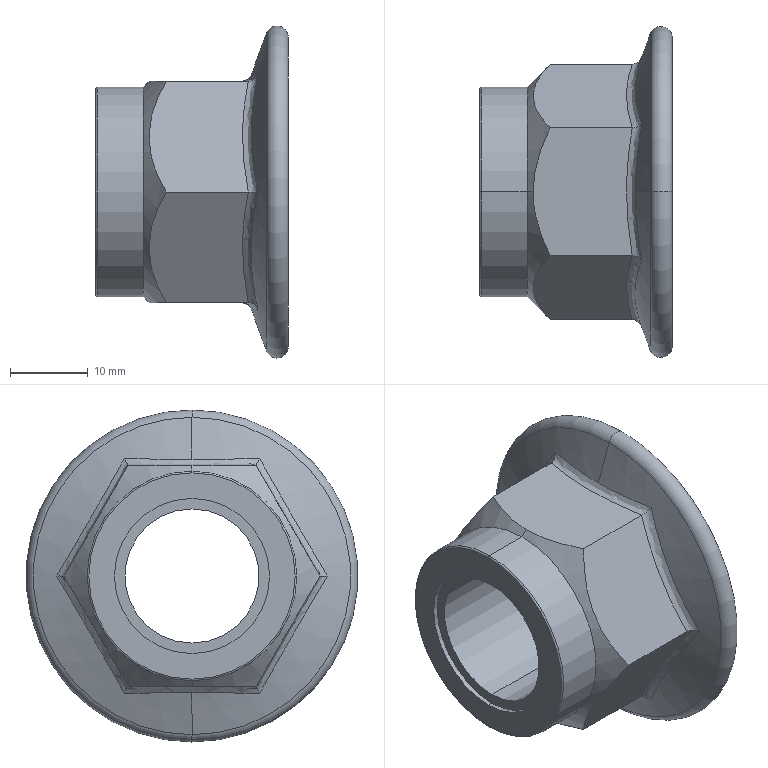Part | SolidWorks | features Cut 2, Revolution 2, Boss 1, Chamfer 1, Fillet 1 | 1 solid | 31 faces | box 24.8 x 42.8 x 42.8 mm | volume 13100 mm3 | plane 9 | cylinder 6 | cone 6 | spline 6 | torus 4 | commonest cylinder face diameters 17.294 x2 20 x2 27 x2
STEP:
#1=CARTESIAN_POINT('',(-24.8,0.,10.));
#2=VERTEX_POINT('',#1);
#3=CARTESIAN_POINT('',(-24.8,0.,-10.));
#4=VERTEX_POINT('',#3);
#5=CARTESIAN_POINT('',(-24.8,0.,0.));
#6=DIRECTION('',(1.,0.,0.));
#7=DIRECTION('',(0.,0.,-1.));
#8=AXIS2_PLACEMENT_3D('',#5,#6,#7);
#9=CIRCLE('',#8,10.);
#10=EDGE_CURVE('',#2,#4,#9,.T.);
#11=ORIENTED_EDGE('',*,*,#10,.F.);
#12=CARTESIAN_POINT('',(-24.19,0.,10.));
#13=VERTEX_POINT('',#12);
#14=CARTESIAN_POINT('',(0.,0.,10.));
#15=DIRECTION('',(1.,0.,0.));
#16=VECTOR('',#15,1000.);
#17=LINE('',#14,#16);
#18=EDGE_CURVE('',#2,#13,#17,.T.);
#19=ORIENTED_EDGE('',*,*,#18,.T.);
#20=CARTESIAN_POINT('',(-24.19,0.,-10.));
#21=VERTEX_POINT('',#20);
#22=CARTESIAN_POINT('',(-24.19,0.,0.));
#23=DIRECTION('',(1.,0.,0.));
#24=DIRECTION('',(0.,0.,-1.));
#25=AXIS2_PLACEMENT_3D('',#22,#23,#24);
#26=CIRCLE('',#25,10.);
#27=EDGE_CURVE('',#13,#21,#26,.T.);
#28=ORIENTED_EDGE('',*,*,#27,.T.);
#29=CARTESIAN_POINT('',(0.,0.,-10.));
#30=DIRECTION('',(1.,0.,0.));
#31=VECTOR('',#30,1000.);
#32=LINE('',#29,#31);
#33=EDGE_CURVE('',#4,#21,#32,.T.);
#34=ORIENTED_EDGE('',*,*,#33,.F.);
#35=EDGE_LOOP('',(#11,#19,#28,#34));
#36=FACE_OUTER_BOUND('',#35,.T.);
#37=CARTESIAN_POINT('',(0.,0.,0.));
#38=DIRECTION('',(1.,0.,0.));
#39=DIRECTION('',(0.,0.,-1.));
#40=AXIS2_PLACEMENT_3D('',#37,#38,#39);
#41=CYLINDRICAL_SURFACE('',#40,10.);
#42=ADVANCED_FACE('',(#36),#41,.F.);
#43=CARTESIAN_POINT('',(-24.8,0.,-13.3));
#44=VERTEX_POINT('',#43);
#45=CARTESIAN_POINT('',(-24.8,0.,13.3));
#46=VERTEX_POINT('',#45);
#47=CARTESIAN_POINT('',(-24.8,0.,0.));
#48=DIRECTION('',(1.,0.,0.));
#49=DIRECTION('',(0.,0.,-1.));
#50=AXIS2_PLACEMENT_3D('',#47,#48,#49);
#51=CIRCLE('',#50,13.3);
#52=EDGE_CURVE('',#44,#46,#51,.T.);
#53=ORIENTED_EDGE('',*,*,#52,.T.);
#54=CARTESIAN_POINT('',(-24.6,0.,13.5));
#55=VERTEX_POINT('',#54);
#56=CARTESIAN_POINT('',(-24.6,0.,13.3));
#57=DIRECTION('',(0.,1.,0.));
#58=DIRECTION('',(0.,0.,1.));
#59=AXIS2_PLACEMENT_3D('',#56,#57,#58);
#60=CIRCLE('',#59,0.2);
#61=EDGE_CURVE('',#46,#55,#60,.T.);
#62=ORIENTED_EDGE('',*,*,#61,.T.);
#63=CARTESIAN_POINT('',(-24.6,0.,-13.5));
#64=VERTEX_POINT('',#63);
#65=CARTESIAN_POINT('',(-24.6,0.,0.));
#66=DIRECTION('',(1.,0.,0.));
#67=DIRECTION('',(0.,0.,-1.));
#68=AXIS2_PLACEMENT_3D('',#65,#66,#67);
#69=CIRCLE('',#68,13.5);
#70=EDGE_CURVE('',#64,#55,#69,.T.);
#71=ORIENTED_EDGE('',*,*,#70,.F.);
#72=CARTESIAN_POINT('',(-24.6,0.,-13.3));
#73=DIRECTION('',(0.,-1.,0.));
#74=DIRECTION('',(0.,0.,-1.));
#75=AXIS2_PLACEMENT_3D('',#72,#73,#74);
#76=CIRCLE('',#75,0.2);
#77=EDGE_CURVE('',#44,#64,#76,.T.);
#78=ORIENTED_EDGE('',*,*,#77,.F.);
#79=EDGE_LOOP('',(#53,#62,#71,#78));
#80=FACE_OUTER_BOUND('',#79,.T.);
#81=CARTESIAN_POINT('',(-24.6,0.,0.));
#82=DIRECTION('',(1.,0.,0.));
#83=DIRECTION('',(0.,0.,-1.));
#84=AXIS2_PLACEMENT_3D('',#81,#82,#83);
#85=TOROIDAL_SURFACE('',#84,13.3,0.2);
#86=ADVANCED_FACE('',(#80),#85,.T.);
#87=ORIENTED_EDGE('',*,*,#70,.T.);
#88=CARTESIAN_POINT('',(-18.7,0.,13.5));
#89=VERTEX_POINT('',#88);
#90=CARTESIAN_POINT('',(0.,0.,13.5));
#91=DIRECTION('',(1.,0.,0.));
#92=VECTOR('',#91,1000.);
#93=LINE('',#90,#92);
#94=EDGE_CURVE('',#55,#89,#93,.T.);
#95=ORIENTED_EDGE('',*,*,#94,.T.);
#96=CARTESIAN_POINT('',(-18.7,0.,-13.5));
#97=VERTEX_POINT('',#96);
#98=CARTESIAN_POINT('',(-18.7,0.,0.));
#99=DIRECTION('',(-1.,0.,0.));
#100=DIRECTION('',(0.,0.,1.));
#101=AXIS2_PLACEMENT_3D('',#98,#99,#100);
#102=CIRCLE('',#101,13.5);
#103=EDGE_CURVE('',#89,#97,#102,.T.);
#104=ORIENTED_EDGE('',*,*,#103,.T.);
#105=CARTESIAN_POINT('',(0.,0.,-13.5));
#106=DIRECTION('',(1.,0.,0.));
#107=VECTOR('',#106,1000.);
#108=LINE('',#105,#107);
#109=EDGE_CURVE('',#64,#97,#108,.T.);
#110=ORIENTED_EDGE('',*,*,#109,.F.);
#111=EDGE_LOOP('',(#87,#95,#104,#110));
#112=FACE_OUTER_BOUND('',#111,.T.);
#113=CARTESIAN_POINT('',(0.,0.,0.));
#114=DIRECTION('',(1.,0.,0.));
#115=DIRECTION('',(0.,0.,-1.));
#116=AXIS2_PLACEMENT_3D('',#113,#114,#115);
#117=CYLINDRICAL_SURFACE('',#116,13.5);
#118=ADVANCED_FACE('',(#112),#117,.T.);
#119=CARTESIAN_POINT('',(-18.7,0.,0.));
#120=DIRECTION('',(-1.,0.,0.));
#121=DIRECTION('',(0.,0.,1.));
#122=AXIS2_PLACEMENT_3D('',#119,#120,#121);
#123=CIRCLE('',#122,13.5);
#124=EDGE_CURVE('',#97,#89,#123,.T.);
#125=ORIENTED_EDGE('',*,*,#124,.F.);
#126=CARTESIAN_POINT('',(-17.932,0.,-14.268));
#127=VERTEX_POINT('',#126);
#128=CARTESIAN_POINT('',(-18.7,0.,-13.5));
#129=DIRECTION('',(0.7071,0.,-0.7071));
#130=VECTOR('',#129,1000.);
#131=LINE('',#128,#130);
#132=EDGE_CURVE('',#97,#127,#131,.T.);
#133=ORIENTED_EDGE('',*,*,#132,.T.);
#134=CARTESIAN_POINT('',(-15.725,-8.238,-14.268));
#135=VERTEX_POINT('',#134);
#136=CARTESIAN_POINT('',(-17.932,0.,-14.268));
#137=CARTESIAN_POINT('',(-17.932,-0.3616,-14.268));
#138=CARTESIAN_POINT('',(-17.918,-0.7252,-14.268));
#139=CARTESIAN_POINT('',(-17.864,-1.443,-14.268));
#140=CARTESIAN_POINT('',(-17.824,-1.799,-14.268));
#141=CARTESIAN_POINT('',(-17.665,-2.859,-14.268));
#142=CARTESIAN_POINT('',(-17.511,-3.555,-14.268));
#143=CARTESIAN_POINT('',(-17.119,-4.928,-14.268));
#144=CARTESIAN_POINT('',(-16.882,-5.607,-14.268));
#145=CARTESIAN_POINT('',(-16.343,-6.947,-14.268));
#146=CARTESIAN_POINT('',(-16.044,-7.599,-14.268));
#147=CARTESIAN_POINT('',(-15.725,-8.238,-14.268));
#148=B_SPLINE_CURVE_WITH_KNOTS('',3,(#136,#137,#138,#139,#140,#141,#142,#143,#144,#145,#146,#147),.UNSPECIFIED.,.F.,.F.,(4,2,2,2,2,4),(0.01727,0.01833,0.0194,0.02153,0.02366,0.0258),.UNSPECIFIED.);
#149=EDGE_CURVE('',#127,#135,#148,.T.);
#150=ORIENTED_EDGE('',*,*,#149,.T.);
#151=CARTESIAN_POINT('',(-15.725,-16.475,0.));
#152=VERTEX_POINT('',#151);
#153=CARTESIAN_POINT('',(-15.725,-8.238,-14.268));
#154=CARTESIAN_POINT('',(-16.369,-8.881,-13.153));
#155=CARTESIAN_POINT('',(-16.916,-9.539,-12.013));
#156=CARTESIAN_POINT('',(-17.502,-10.562,-10.242));
#157=CARTESIAN_POINT('',(-17.658,-10.909,-9.641));
#158=CARTESIAN_POINT('',(-17.873,-11.617,-8.415));
#159=CARTESIAN_POINT('',(-17.931,-11.982,-7.783));
#160=CARTESIAN_POINT('',(-17.935,-13.06,-5.915));
#161=CARTESIAN_POINT('',(-17.717,-13.767,-4.69));
#162=CARTESIAN_POINT('',(-16.928,-15.161,-2.276));
#163=CARTESIAN_POINT('',(-16.372,-15.828,-1.121));
#164=CARTESIAN_POINT('',(-15.725,-16.475,0.));
#165=B_SPLINE_CURVE_WITH_KNOTS('',3,(#153,#154,#155,#156,#157,#158,#159,#160,#161,#162,#163,#164),.UNSPECIFIED.,.F.,.F.,(4,2,2,2,2,4),(0.000000254,0.004255,0.006382,0.008509,0.01276,0.01702),.UNSPECIFIED.);
#166=EDGE_CURVE('',#135,#152,#165,.T.);
#167=ORIENTED_EDGE('',*,*,#166,.T.);
#168=CARTESIAN_POINT('',(-15.725,-8.238,14.268));
#169=VERTEX_POINT('',#168);
#170=CARTESIAN_POINT('',(-15.725,-16.475,0.));
#171=CARTESIAN_POINT('',(-16.369,-15.831,1.115));
#172=CARTESIAN_POINT('',(-16.916,-15.173,2.255));
#173=CARTESIAN_POINT('',(-17.502,-14.151,4.026));
#174=CARTESIAN_POINT('',(-17.658,-13.804,4.626));
#175=CARTESIAN_POINT('',(-17.873,-13.096,5.853));
#176=CARTESIAN_POINT('',(-17.931,-12.731,6.485));
#177=CARTESIAN_POINT('',(-17.935,-11.652,8.353));
#178=CARTESIAN_POINT('',(-17.717,-10.945,9.577));
#179=CARTESIAN_POINT('',(-16.928,-9.552,11.992));
#180=CARTESIAN_POINT('',(-16.372,-8.885,13.146));
#181=CARTESIAN_POINT('',(-15.725,-8.238,14.268));
#182=B_SPLINE_CURVE_WITH_KNOTS('',3,(#170,#171,#172,#173,#174,#175,#176,#177,#178,#179,#180,#181),.UNSPECIFIED.,.F.,.F.,(4,2,2,2,2,4),(0.000000254,0.004255,0.006382,0.008509,0.01276,0.01702),.UNSPECIFIED.);
#183=EDGE_CURVE('',#152,#169,#182,.T.);
#184=ORIENTED_EDGE('',*,*,#183,.T.);
#185=CARTESIAN_POINT('',(-17.932,0.,14.268));
#186=VERTEX_POINT('',#185);
#187=CARTESIAN_POINT('',(-15.725,-8.238,14.268));
#188=CARTESIAN_POINT('',(-16.044,-7.599,14.268));
#189=CARTESIAN_POINT('',(-16.343,-6.947,14.268));
#190=CARTESIAN_POINT('',(-16.882,-5.607,14.268));
#191=CARTESIAN_POINT('',(-17.119,-4.928,14.268));
#192=CARTESIAN_POINT('',(-17.511,-3.555,14.268));
#193=CARTESIAN_POINT('',(-17.665,-2.859,14.268));
#194=CARTESIAN_POINT('',(-17.824,-1.799,14.268));
#195=CARTESIAN_POINT('',(-17.864,-1.443,14.268));
#196=CARTESIAN_POINT('',(-17.918,-0.7252,14.268));
#197=CARTESIAN_POINT('',(-17.932,-0.3616,14.268));
#198=CARTESIAN_POINT('',(-17.932,0.,14.268));
#199=B_SPLINE_CURVE_WITH_KNOTS('',3,(#187,#188,#189,#190,#191,#192,#193,#194,#195,#196,#197,#198),.UNSPECIFIED.,.F.,.F.,(4,2,2,2,2,4),(0.01093,0.01306,0.0152,0.01733,0.0184,0.01946),.UNSPECIFIED.);
#200=EDGE_CURVE('',#169,#186,#199,.T.);
#201=ORIENTED_EDGE('',*,*,#200,.T.);
#202=CARTESIAN_POINT('',(-18.7,0.,13.5));
#203=DIRECTION('',(0.7071,0.,0.7071));
#204=VECTOR('',#203,1000.);
#205=LINE('',#202,#204);
#206=EDGE_CURVE('',#89,#186,#205,.T.);
#207=ORIENTED_EDGE('',*,*,#206,.F.);
#208=EDGE_LOOP('',(#125,#133,#150,#167,#184,#201,#207));
#209=FACE_OUTER_BOUND('',#208,.T.);
#210=CARTESIAN_POINT('',(-18.7,0.,0.));
#211=DIRECTION('',(1.,0.,0.));
#212=DIRECTION('',(0.,0.,1.));
#213=AXIS2_PLACEMENT_3D('',#210,#211,#212);
#214=CONICAL_SURFACE('',#213,13.5,0.7854);
#215=ADVANCED_FACE('',(#209),#214,.T.);
#216=CARTESIAN_POINT('',(-2.153,0.,8.647));
#217=VERTEX_POINT('',#216);
#218=CARTESIAN_POINT('',(-2.153,0.,-8.647));
#219=VERTEX_POINT('',#218);
#220=CARTESIAN_POINT('',(-2.153,0.,0.));
#221=DIRECTION('',(1.,0.,0.));
#222=DIRECTION('',(0.,0.,1.));
#223=AXIS2_PLACEMENT_3D('',#220,#221,#222);
#224=CIRCLE('',#223,8.647);
#225=EDGE_CURVE('',#217,#219,#224,.T.);
#226=ORIENTED_EDGE('',*,*,#225,.F.);
#227=CARTESIAN_POINT('',(0.,0.,10.8));
#228=VERTEX_POINT('',#227);
#229=CARTESIAN_POINT('',(0.,0.,10.8));
#230=DIRECTION('',(0.7071,0.,0.7071));
#231=VECTOR('',#230,1000.);
#232=LINE('',#229,#231);
#233=EDGE_CURVE('',#217,#228,#232,.T.);
#234=ORIENTED_EDGE('',*,*,#233,.T.);
#235=CARTESIAN_POINT('',(0.,0.,-10.8));
#236=VERTEX_POINT('',#235);
#237=CARTESIAN_POINT('',(0.,0.,0.));
#238=DIRECTION('',(-1.,0.,0.));
#239=DIRECTION('',(0.,0.,1.));
#240=AXIS2_PLACEMENT_3D('',#237,#238,#239);
#241=CIRCLE('',#240,10.8);
#242=EDGE_CURVE('',#236,#228,#241,.T.);
#243=ORIENTED_EDGE('',*,*,#242,.F.);
#244=CARTESIAN_POINT('',(0.,0.,-10.8));
#245=DIRECTION('',(0.7071,0.,-0.7071));
#246=VECTOR('',#245,1000.);
#247=LINE('',#244,#246);
#248=EDGE_CURVE('',#219,#236,#247,.T.);
#249=ORIENTED_EDGE('',*,*,#248,.F.);
#250=EDGE_LOOP('',(#226,#234,#243,#249));
#251=FACE_OUTER_BOUND('',#250,.T.);
#252=CARTESIAN_POINT('',(0.,0.,0.));
#253=DIRECTION('',(1.,0.,0.));
#254=DIRECTION('',(0.,0.,-1.));
#255=AXIS2_PLACEMENT_3D('',#252,#253,#254);
#256=CONICAL_SURFACE('',#255,10.8,0.7854);
#257=ADVANCED_FACE('',(#251),#256,.F.);
#258=ORIENTED_EDGE('',*,*,#225,.T.);
#259=CARTESIAN_POINT('',(-24.19,0.,-8.647));
#260=VERTEX_POINT('',#259);
#261=CARTESIAN_POINT('',(0.,0.,-8.647));
#262=DIRECTION('',(-1.,0.,0.));
#263=VECTOR('',#262,1000.);
#264=LINE('',#261,#263);
#265=EDGE_CURVE('',#219,#260,#264,.T.);
#266=ORIENTED_EDGE('',*,*,#265,.T.);
#267=CARTESIAN_POINT('',(-24.19,0.,8.647));
#268=VERTEX_POINT('',#267);
#269=CARTESIAN_POINT('',(-24.19,0.,0.));
#270=DIRECTION('',(1.,0.,0.));
#271=DIRECTION('',(0.,0.,-1.));
#272=AXIS2_PLACEMENT_3D('',#269,#270,#271);
#273=CIRCLE('',#272,8.647);
#274=EDGE_CURVE('',#268,#260,#273,.T.);
#275=ORIENTED_EDGE('',*,*,#274,.F.);
#276=CARTESIAN_POINT('',(0.,0.,8.647));
#277=DIRECTION('',(-1.,0.,0.));
#278=VECTOR('',#277,1000.);
#279=LINE('',#276,#278);
#280=EDGE_CURVE('',#217,#268,#279,.T.);
#281=ORIENTED_EDGE('',*,*,#280,.F.);
#282=EDGE_LOOP('',(#258,#266,#275,#281));
#283=FACE_OUTER_BOUND('',#282,.T.);
#284=CARTESIAN_POINT('',(0.,0.,0.));
#285=DIRECTION('',(-1.,0.,0.));
#286=DIRECTION('',(0.,0.,1.));
#287=AXIS2_PLACEMENT_3D('',#284,#285,#286);
#288=CYLINDRICAL_SURFACE('',#287,8.647);
#289=ADVANCED_FACE('',(#283),#288,.F.);
#290=CARTESIAN_POINT('',(0.,0.,19.95));
#291=VERTEX_POINT('',#290);
#292=CARTESIAN_POINT('',(0.,0.,-19.95));
#293=VERTEX_POINT('',#292);
#294=CARTESIAN_POINT('',(0.,0.,0.));
#295=DIRECTION('',(-1.,0.,0.));
#296=DIRECTION('',(0.,0.,1.));
#297=AXIS2_PLACEMENT_3D('',#294,#295,#296);
#298=CIRCLE('',#297,19.95);
#299=EDGE_CURVE('',#291,#293,#298,.T.);
#300=ORIENTED_EDGE('',*,*,#299,.T.);
#301=CARTESIAN_POINT('',(-2.813,0.,-20.446));
#302=VERTEX_POINT('',#301);
#303=CARTESIAN_POINT('',(-1.45,0.,-19.95));
#304=DIRECTION('',(0.,1.,0.));
#305=DIRECTION('',(0.,0.,1.));
#306=AXIS2_PLACEMENT_3D('',#303,#304,#305);
#307=CIRCLE('',#306,1.45);
#308=EDGE_CURVE('',#293,#302,#307,.T.);
#309=ORIENTED_EDGE('',*,*,#308,.T.);
#310=CARTESIAN_POINT('',(-2.813,0.,20.446));
#311=VERTEX_POINT('',#310);
#312=CARTESIAN_POINT('',(-2.813,0.,0.));
#313=DIRECTION('',(-1.,0.,0.));
#314=DIRECTION('',(0.,0.,1.));
#315=AXIS2_PLACEMENT_3D('',#312,#313,#314);
#316=CIRCLE('',#315,20.446);
#317=EDGE_CURVE('',#311,#302,#316,.T.);
#318=ORIENTED_EDGE('',*,*,#317,.F.);
#319=CARTESIAN_POINT('',(-1.45,0.,19.95));
#320=DIRECTION('',(0.,-1.,0.));
#321=DIRECTION('',(0.,0.,-1.));
#322=AXIS2_PLACEMENT_3D('',#319,#320,#321);
#323=CIRCLE('',#322,1.45);
#324=EDGE_CURVE('',#291,#311,#323,.T.);
#325=ORIENTED_EDGE('',*,*,#324,.F.);
#326=EDGE_LOOP('',(#300,#309,#318,#325));
#327=FACE_OUTER_BOUND('',#326,.T.);
#328=CARTESIAN_POINT('',(-1.45,0.,0.));
#329=DIRECTION('',(-1.,0.,0.));
#330=DIRECTION('',(0.,0.,1.));
#331=AXIS2_PLACEMENT_3D('',#328,#329,#330);
#332=TOROIDAL_SURFACE('',#331,19.95,1.45);
#333=ADVANCED_FACE('',(#327),#332,.T.);
#334=CARTESIAN_POINT('',(-3.903,8.725,15.112));
#335=VERTEX_POINT('',#334);
#336=CARTESIAN_POINT('',(-4.774,0.,15.057));
#337=VERTEX_POINT('',#336);
#338=CARTESIAN_POINT('',(-3.903,8.725,15.112));
#339=CARTESIAN_POINT('',(-4.17,7.283,15.098));
#340=CARTESIAN_POINT('',(-4.389,5.836,15.084));
#341=CARTESIAN_POINT('',(-4.692,2.929,15.063));
#342=CARTESIAN_POINT('',(-4.774,1.469,15.057));
#343=CARTESIAN_POINT('',(-4.774,0.,15.057));
#344=B_SPLINE_CURVE_WITH_KNOTS('',3,(#338,#339,#340,#341,#342,#343),.UNSPECIFIED.,.F.,.F.,(4,2,4),(0.,0.004384,0.008769),.UNSPECIFIED.);
#345=EDGE_CURVE('',#335,#337,#344,.T.);
#346=ORIENTED_EDGE('',*,*,#345,.T.);
#347=CARTESIAN_POINT('',(-2.813,0.,20.446));
#348=DIRECTION('',(0.342,0.,0.9397));
#349=VECTOR('',#348,1000.);
#350=LINE('',#347,#349);
#351=EDGE_CURVE('',#337,#311,#350,.T.);
#352=ORIENTED_EDGE('',*,*,#351,.T.);
#353=ORIENTED_EDGE('',*,*,#317,.T.);
#354=CARTESIAN_POINT('',(-4.774,0.,-15.057));
#355=VERTEX_POINT('',#354);
#356=CARTESIAN_POINT('',(-2.813,0.,-20.446));
#357=DIRECTION('',(0.342,0.,-0.9397));
#358=VECTOR('',#357,1000.);
#359=LINE('',#356,#358);
#360=EDGE_CURVE('',#355,#302,#359,.T.);
#361=ORIENTED_EDGE('',*,*,#360,.F.);
#362=CARTESIAN_POINT('',(-3.903,8.725,-15.112));
#363=VERTEX_POINT('',#362);
#364=CARTESIAN_POINT('',(-4.774,0.,-15.057));
#365=CARTESIAN_POINT('',(-4.774,1.465,-15.057));
#366=CARTESIAN_POINT('',(-4.692,2.925,-15.063));
#367=CARTESIAN_POINT('',(-4.389,5.839,-15.084));
#368=CARTESIAN_POINT('',(-4.17,7.285,-15.098));
#369=CARTESIAN_POINT('',(-3.903,8.725,-15.112));
#370=B_SPLINE_CURVE_WITH_KNOTS('',3,(#364,#365,#366,#367,#368,#369),.UNSPECIFIED.,.F.,.F.,(4,2,4),(0.008769,0.01314,0.01751),.UNSPECIFIED.);
#371=EDGE_CURVE('',#355,#363,#370,.T.);
#372=ORIENTED_EDGE('',*,*,#371,.T.);
#373=CARTESIAN_POINT('',(-3.903,17.45,0.));
#374=VERTEX_POINT('',#373);
#375=CARTESIAN_POINT('',(-3.903,8.725,-15.112));
#376=CARTESIAN_POINT('',(-4.17,9.433,-13.858));
#377=CARTESIAN_POINT('',(-4.389,10.143,-12.6));
#378=CARTESIAN_POINT('',(-4.691,11.577,-10.075));
#379=CARTESIAN_POINT('',(-4.773,12.301,-8.809));
#380=CARTESIAN_POINT('',(-4.774,13.767,-6.269));
#381=CARTESIAN_POINT('',(-4.693,14.504,-5.005));
#382=CARTESIAN_POINT('',(-4.39,15.98,-2.489));
#383=CARTESIAN_POINT('',(-4.17,16.717,-1.241));
#384=CARTESIAN_POINT('',(-3.903,17.45,0.));
#385=B_SPLINE_CURVE_WITH_KNOTS('',3,(#375,#376,#377,#378,#379,#380,#381,#382,#383,#384),.UNSPECIFIED.,.F.,.F.,(4,2,2,2,4),(0.,0.004378,0.008757,0.01314,0.01751),.UNSPECIFIED.);
#386=EDGE_CURVE('',#363,#374,#385,.T.);
#387=ORIENTED_EDGE('',*,*,#386,.T.);
#388=CARTESIAN_POINT('',(-3.903,17.45,0.));
#389=CARTESIAN_POINT('',(-4.17,16.718,1.24));
#390=CARTESIAN_POINT('',(-4.389,15.983,2.484));
#391=CARTESIAN_POINT('',(-4.691,14.514,4.988));
#392=CARTESIAN_POINT('',(-4.773,13.779,6.248));
#393=CARTESIAN_POINT('',(-4.774,12.313,8.789));
#394=CARTESIAN_POINT('',(-4.693,11.587,10.058));
#395=CARTESIAN_POINT('',(-4.39,10.146,12.595));
#396=CARTESIAN_POINT('',(-4.17,9.433,13.856));
#397=CARTESIAN_POINT('',(-3.903,8.725,15.112));
#398=B_SPLINE_CURVE_WITH_KNOTS('',3,(#388,#389,#390,#391,#392,#393,#394,#395,#396,#397),.UNSPECIFIED.,.F.,.F.,(4,2,2,2,4),(0.,0.004378,0.008757,0.01314,0.01751),.UNSPECIFIED.);
#399=EDGE_CURVE('',#374,#335,#398,.T.);
#400=ORIENTED_EDGE('',*,*,#399,.T.);
#401=EDGE_LOOP('',(#346,#352,#353,#361,#372,#387,#400));
#402=FACE_OUTER_BOUND('',#401,.T.);
#403=CARTESIAN_POINT('',(-2.813,0.,0.));
#404=DIRECTION('',(1.,0.,0.));
#405=DIRECTION('',(0.,0.,-1.));
#406=AXIS2_PLACEMENT_3D('',#403,#404,#405);
#407=CONICAL_SURFACE('',#406,20.446,1.222);
#408=ADVANCED_FACE('',(#402),#407,.T.);
#409=CARTESIAN_POINT('',(-15.725,8.238,14.268));
#410=VERTEX_POINT('',#409);
#411=CARTESIAN_POINT('',(-5.153,8.238,14.268));
#412=VERTEX_POINT('',#411);
#413=CARTESIAN_POINT('',(-18.7,8.238,14.268));
#414=DIRECTION('',(1.,0.,0.));
#415=VECTOR('',#414,1000.);
#416=LINE('',#413,#415);
#417=EDGE_CURVE('',#410,#412,#416,.T.);
#418=ORIENTED_EDGE('',*,*,#417,.T.);
#419=CARTESIAN_POINT('',(-5.153,16.475,0.));
#420=VERTEX_POINT('',#419);
#421=CARTESIAN_POINT('',(-5.153,8.238,14.268));
#422=CARTESIAN_POINT('',(-5.386,8.919,13.087));
#423=CARTESIAN_POINT('',(-5.575,9.603,11.903));
#424=CARTESIAN_POINT('',(-5.833,10.975,9.526));
#425=CARTESIAN_POINT('',(-5.901,11.664,8.333));
#426=CARTESIAN_POINT('',(-5.901,13.048,5.935));
#427=CARTESIAN_POINT('',(-5.833,13.737,4.742));
#428=CARTESIAN_POINT('',(-5.575,15.11,2.364));
#429=CARTESIAN_POINT('',(-5.386,15.793,1.18));
#430=CARTESIAN_POINT('',(-5.153,16.475,0.));
#431=B_SPLINE_CURVE_WITH_KNOTS('',3,(#421,#422,#423,#424,#425,#426,#427,#428,#429,#430),.UNSPECIFIED.,.F.,.F.,(4,2,2,2,4),(0.,0.004136,0.008271,0.01241,0.01654),.UNSPECIFIED.);
#432=EDGE_CURVE('',#412,#420,#431,.T.);
#433=ORIENTED_EDGE('',*,*,#432,.T.);
#434=CARTESIAN_POINT('',(-15.725,16.475,0.));
#435=VERTEX_POINT('',#434);
#436=CARTESIAN_POINT('',(-18.7,16.475,0.));
#437=DIRECTION('',(1.,0.,0.));
#438=VECTOR('',#437,1000.);
#439=LINE('',#436,#438);
#440=EDGE_CURVE('',#435,#420,#439,.T.);
#441=ORIENTED_EDGE('',*,*,#440,.F.);
#442=CARTESIAN_POINT('',(-15.725,8.238,14.268));
#443=CARTESIAN_POINT('',(-16.369,8.881,13.153));
#444=CARTESIAN_POINT('',(-16.916,9.539,12.013));
#445=CARTESIAN_POINT('',(-17.502,10.562,10.242));
#446=CARTESIAN_POINT('',(-17.658,10.909,9.641));
#447=CARTESIAN_POINT('',(-17.873,11.617,8.415));
#448=CARTESIAN_POINT('',(-17.931,11.982,7.783));
#449=CARTESIAN_POINT('',(-17.935,13.06,5.915));
#450=CARTESIAN_POINT('',(-17.717,13.767,4.69));
#451=CARTESIAN_POINT('',(-16.928,15.161,2.276));
#452=CARTESIAN_POINT('',(-16.372,15.828,1.121));
#453=CARTESIAN_POINT('',(-15.725,16.475,0.));
#454=B_SPLINE_CURVE_WITH_KNOTS('',3,(#442,#443,#444,#445,#446,#447,#448,#449,#450,#451,#452,#453),.UNSPECIFIED.,.F.,.F.,(4,2,2,2,2,4),(0.000000254,0.004255,0.006382,0.008509,0.01276,0.01702),.UNSPECIFIED.);
#455=EDGE_CURVE('',#410,#435,#454,.T.);
#456=ORIENTED_EDGE('',*,*,#455,.F.);
#457=EDGE_LOOP('',(#418,#433,#441,#456));
#458=FACE_OUTER_BOUND('',#457,.T.);
#459=CARTESIAN_POINT('',(-18.7,8.238,14.268));
#460=DIRECTION('',(0.,-0.866,-0.5));
#461=DIRECTION('',(0.,0.5,-0.866));
#462=AXIS2_PLACEMENT_3D('',#459,#460,#461);
#463=PLANE('',#462);
#464=ADVANCED_FACE('',(#458),#463,.F.);
#465=ORIENTED_EDGE('',*,*,#440,.T.);
#466=CARTESIAN_POINT('',(-5.153,8.238,-14.268));
#467=VERTEX_POINT('',#466);
#468=CARTESIAN_POINT('',(-5.153,16.475,0.));
#469=CARTESIAN_POINT('',(-5.386,15.793,-1.18));
#470=CARTESIAN_POINT('',(-5.575,15.11,-2.364));
#471=CARTESIAN_POINT('',(-5.833,13.737,-4.742));
#472=CARTESIAN_POINT('',(-5.901,13.048,-5.935));
#473=CARTESIAN_POINT('',(-5.901,11.664,-8.333));
#474=CARTESIAN_POINT('',(-5.833,10.975,-9.526));
#475=CARTESIAN_POINT('',(-5.575,9.603,-11.903));
#476=CARTESIAN_POINT('',(-5.386,8.919,-13.087));
#477=CARTESIAN_POINT('',(-5.153,8.238,-14.268));
#478=B_SPLINE_CURVE_WITH_KNOTS('',3,(#468,#469,#470,#471,#472,#473,#474,#475,#476,#477),.UNSPECIFIED.,.F.,.F.,(4,2,2,2,4),(0.,0.004136,0.008271,0.01241,0.01654),.UNSPECIFIED.);
#479=EDGE_CURVE('',#420,#467,#478,.T.);
#480=ORIENTED_EDGE('',*,*,#479,.T.);
#481=CARTESIAN_POINT('',(-15.725,8.238,-14.268));
#482=VERTEX_POINT('',#481);
#483=CARTESIAN_POINT('',(-18.7,8.238,-14.268));
#484=DIRECTION('',(1.,0.,0.));
#485=VECTOR('',#484,1000.);
#486=LINE('',#483,#485);
#487=EDGE_CURVE('',#482,#467,#486,.T.);
#488=ORIENTED_EDGE('',*,*,#487,.F.);
#489=CARTESIAN_POINT('',(-15.725,16.475,0.));
#490=CARTESIAN_POINT('',(-16.369,15.831,-1.115));
#491=CARTESIAN_POINT('',(-16.916,15.173,-2.255));
#492=CARTESIAN_POINT('',(-17.502,14.151,-4.026));
#493=CARTESIAN_POINT('',(-17.658,13.804,-4.626));
#494=CARTESIAN_POINT('',(-17.873,13.096,-5.853));
#495=CARTESIAN_POINT('',(-17.931,12.731,-6.485));
#496=CARTESIAN_POINT('',(-17.935,11.652,-8.353));
#497=CARTESIAN_POINT('',(-17.717,10.945,-9.577));
#498=CARTESIAN_POINT('',(-16.928,9.552,-11.992));
#499=CARTESIAN_POINT('',(-16.372,8.885,-13.146));
#500=CARTESIAN_POINT('',(-15.725,8.238,-14.268));
#501=B_SPLINE_CURVE_WITH_KNOTS('',3,(#489,#490,#491,#492,#493,#494,#495,#496,#497,#498,#499,#500),.UNSPECIFIED.,.F.,.F.,(4,2,2,2,2,4),(0.000000254,0.004255,0.006382,0.008509,0.01276,0.01702),.UNSPECIFIED.);
#502=EDGE_CURVE('',#435,#482,#501,.T.);
#503=ORIENTED_EDGE('',*,*,#502,.F.);
#504=EDGE_LOOP('',(#465,#480,#488,#503));
#505=FACE_OUTER_BOUND('',#504,.T.);
#506=CARTESIAN_POINT('',(-18.7,16.475,0.));
#507=DIRECTION('',(0.,-0.866,0.5));
#508=DIRECTION('',(0.,-0.5,-0.866));
#509=AXIS2_PLACEMENT_3D('',#506,#507,#508);
#510=PLANE('',#509);
#511=ADVANCED_FACE('',(#505),#510,.F.);
#512=ORIENTED_EDGE('',*,*,#487,.T.);
#513=CARTESIAN_POINT('',(-5.153,-8.238,-14.268));
#514=VERTEX_POINT('',#513);
#515=CARTESIAN_POINT('',(-5.153,8.238,-14.268));
#516=CARTESIAN_POINT('',(-5.386,6.874,-14.268));
#517=CARTESIAN_POINT('',(-5.575,5.507,-14.268));
#518=CARTESIAN_POINT('',(-5.833,2.762,-14.268));
#519=CARTESIAN_POINT('',(-5.901,1.384,-14.268));
#520=CARTESIAN_POINT('',(-5.901,-1.384,-14.268));
#521=CARTESIAN_POINT('',(-5.833,-2.762,-14.268));
#522=CARTESIAN_POINT('',(-5.575,-5.507,-14.268));
#523=CARTESIAN_POINT('',(-5.386,-6.874,-14.268));
#524=CARTESIAN_POINT('',(-5.153,-8.238,-14.268));
#525=B_SPLINE_CURVE_WITH_KNOTS('',3,(#515,#516,#517,#518,#519,#520,#521,#522,#523,#524),.UNSPECIFIED.,.F.,.F.,(4,2,2,2,4),(0.,0.004136,0.008272,0.01241,0.01654),.UNSPECIFIED.);
#526=EDGE_CURVE('',#467,#514,#525,.T.);
#527=ORIENTED_EDGE('',*,*,#526,.T.);
#528=CARTESIAN_POINT('',(-18.7,-8.238,-14.268));
#529=DIRECTION('',(1.,0.,0.));
#530=VECTOR('',#529,1000.);
#531=LINE('',#528,#530);
#532=EDGE_CURVE('',#135,#514,#531,.T.);
#533=ORIENTED_EDGE('',*,*,#532,.F.);
#534=ORIENTED_EDGE('',*,*,#149,.F.);
#535=CARTESIAN_POINT('',(-15.725,8.238,-14.268));
#536=CARTESIAN_POINT('',(-16.044,7.6,-14.268));
#537=CARTESIAN_POINT('',(-16.341,6.95,-14.268));
#538=CARTESIAN_POINT('',(-16.879,5.617,-14.268));
#539=CARTESIAN_POINT('',(-17.119,4.93,-14.268));
#540=CARTESIAN_POINT('',(-17.709,2.858,-14.268));
#541=CARTESIAN_POINT('',(-17.932,1.448,-14.268));
#542=CARTESIAN_POINT('',(-17.932,0.,-14.268));
#543=B_SPLINE_CURVE_WITH_KNOTS('',3,(#535,#536,#537,#538,#539,#540,#541,#542),.UNSPECIFIED.,.F.,.F.,(4,2,2,4),(0.008726,0.01086,0.013,0.01727),.UNSPECIFIED.);
#544=EDGE_CURVE('',#482,#127,#543,.T.);
#545=ORIENTED_EDGE('',*,*,#544,.F.);
#546=EDGE_LOOP('',(#512,#527,#533,#534,#545));
#547=FACE_OUTER_BOUND('',#546,.T.);
#548=CARTESIAN_POINT('',(-18.7,8.238,-14.268));
#549=DIRECTION('',(0.,0.,1.));
#550=DIRECTION('',(1.,0.,0.));
#551=AXIS2_PLACEMENT_3D('',#548,#549,#550);
#552=PLANE('',#551);
#553=ADVANCED_FACE('',(#547),#552,.F.);
#554=ORIENTED_EDGE('',*,*,#532,.T.);
#555=CARTESIAN_POINT('',(-5.153,-16.475,0.));
#556=VERTEX_POINT('',#555);
#557=CARTESIAN_POINT('',(-5.153,-8.238,-14.268));
#558=CARTESIAN_POINT('',(-5.386,-8.919,-13.087));
#559=CARTESIAN_POINT('',(-5.575,-9.603,-11.903));
#560=CARTESIAN_POINT('',(-5.833,-10.975,-9.526));
#561=CARTESIAN_POINT('',(-5.901,-11.664,-8.333));
#562=CARTESIAN_POINT('',(-5.901,-13.048,-5.935));
#563=CARTESIAN_POINT('',(-5.833,-13.737,-4.742));
#564=CARTESIAN_POINT('',(-5.575,-15.11,-2.364));
#565=CARTESIAN_POINT('',(-5.386,-15.793,-1.18));
#566=CARTESIAN_POINT('',(-5.153,-16.475,0.));
#567=B_SPLINE_CURVE_WITH_KNOTS('',3,(#557,#558,#559,#560,#561,#562,#563,#564,#565,#566),.UNSPECIFIED.,.F.,.F.,(4,2,2,2,4),(0.,0.004136,0.008271,0.01241,0.01654),.UNSPECIFIED.);
#568=EDGE_CURVE('',#514,#556,#567,.T.);
#569=ORIENTED_EDGE('',*,*,#568,.T.);
#570=CARTESIAN_POINT('',(-18.7,-16.475,0.));
#571=DIRECTION('',(1.,0.,0.));
#572=VECTOR('',#571,1000.);
#573=LINE('',#570,#572);
#574=EDGE_CURVE('',#152,#556,#573,.T.);
#575=ORIENTED_EDGE('',*,*,#574,.F.);
#576=ORIENTED_EDGE('',*,*,#166,.F.);
#577=EDGE_LOOP('',(#554,#569,#575,#576));
#578=FACE_OUTER_BOUND('',#577,.T.);
#579=CARTESIAN_POINT('',(-18.7,-8.238,-14.268));
#580=DIRECTION('',(0.,0.866,0.5));
#581=DIRECTION('',(0.,-0.5,0.866));
#582=AXIS2_PLACEMENT_3D('',#579,#580,#581);
#583=PLANE('',#582);
#584=ADVANCED_FACE('',(#578),#583,.F.);
#585=ORIENTED_EDGE('',*,*,#574,.T.);
#586=CARTESIAN_POINT('',(-5.153,-8.238,14.268));
#587=VERTEX_POINT('',#586);
#588=CARTESIAN_POINT('',(-5.153,-16.475,0.));
#589=CARTESIAN_POINT('',(-5.386,-15.793,1.18));
#590=CARTESIAN_POINT('',(-5.575,-15.11,2.364));
#591=CARTESIAN_POINT('',(-5.833,-13.737,4.742));
#592=CARTESIAN_POINT('',(-5.901,-13.048,5.935));
#593=CARTESIAN_POINT('',(-5.901,-11.664,8.333));
#594=CARTESIAN_POINT('',(-5.833,-10.975,9.526));
#595=CARTESIAN_POINT('',(-5.575,-9.603,11.903));
#596=CARTESIAN_POINT('',(-5.386,-8.919,13.087));
#597=CARTESIAN_POINT('',(-5.153,-8.238,14.268));
#598=B_SPLINE_CURVE_WITH_KNOTS('',3,(#588,#589,#590,#591,#592,#593,#594,#595,#596,#597),.UNSPECIFIED.,.F.,.F.,(4,2,2,2,4),(0.,0.004136,0.008271,0.01241,0.01654),.UNSPECIFIED.);
#599=EDGE_CURVE('',#556,#587,#598,.T.);
#600=ORIENTED_EDGE('',*,*,#599,.T.);
#601=CARTESIAN_POINT('',(-18.7,-8.238,14.268));
#602=DIRECTION('',(1.,0.,0.));
#603=VECTOR('',#602,1000.);
#604=LINE('',#601,#603);
#605=EDGE_CURVE('',#169,#587,#604,.T.);
#606=ORIENTED_EDGE('',*,*,#605,.F.);
#607=ORIENTED_EDGE('',*,*,#183,.F.);
#608=EDGE_LOOP('',(#585,#600,#606,#607));
#609=FACE_OUTER_BOUND('',#608,.T.);
#610=CARTESIAN_POINT('',(-18.7,-16.475,0.));
#611=DIRECTION('',(0.,0.866,-0.5));
#612=DIRECTION('',(0.,0.5,0.866));
#613=AXIS2_PLACEMENT_3D('',#610,#611,#612);
#614=PLANE('',#613);
#615=ADVANCED_FACE('',(#609),#614,.F.);
#616=ORIENTED_EDGE('',*,*,#605,.T.);
#617=CARTESIAN_POINT('',(-5.153,-8.238,14.268));
#618=CARTESIAN_POINT('',(-5.386,-6.874,14.268));
#619=CARTESIAN_POINT('',(-5.575,-5.507,14.268));
#620=CARTESIAN_POINT('',(-5.833,-2.762,14.268));
#621=CARTESIAN_POINT('',(-5.901,-1.384,14.268));
#622=CARTESIAN_POINT('',(-5.901,1.384,14.268));
#623=CARTESIAN_POINT('',(-5.833,2.762,14.268));
#624=CARTESIAN_POINT('',(-5.575,5.507,14.268));
#625=CARTESIAN_POINT('',(-5.386,6.874,14.268));
#626=CARTESIAN_POINT('',(-5.153,8.238,14.268));
#627=B_SPLINE_CURVE_WITH_KNOTS('',3,(#617,#618,#619,#620,#621,#622,#623,#624,#625,#626),.UNSPECIFIED.,.F.,.F.,(4,2,2,2,4),(0.,0.004136,0.008271,0.01241,0.01654),.UNSPECIFIED.);
#628=EDGE_CURVE('',#587,#412,#627,.T.);
#629=ORIENTED_EDGE('',*,*,#628,.T.);
#630=ORIENTED_EDGE('',*,*,#417,.F.);
#631=CARTESIAN_POINT('',(-17.932,0.,14.268));
#632=CARTESIAN_POINT('',(-17.932,1.448,14.268));
#633=CARTESIAN_POINT('',(-17.709,2.858,14.268));
#634=CARTESIAN_POINT('',(-17.119,4.93,14.268));
#635=CARTESIAN_POINT('',(-16.879,5.617,14.268));
#636=CARTESIAN_POINT('',(-16.341,6.95,14.268));
#637=CARTESIAN_POINT('',(-16.044,7.6,14.268));
#638=CARTESIAN_POINT('',(-15.725,8.238,14.268));
#639=B_SPLINE_CURVE_WITH_KNOTS('',3,(#631,#632,#633,#634,#635,#636,#637,#638),.UNSPECIFIED.,.F.,.F.,(4,2,2,4),(0.01946,0.02374,0.02587,0.02801),.UNSPECIFIED.);
#640=EDGE_CURVE('',#186,#410,#639,.T.);
#641=ORIENTED_EDGE('',*,*,#640,.F.);
#642=ORIENTED_EDGE('',*,*,#200,.F.);
#643=EDGE_LOOP('',(#616,#629,#630,#641,#642));
#644=FACE_OUTER_BOUND('',#643,.T.);
#645=CARTESIAN_POINT('',(-18.7,-8.238,14.268));
#646=DIRECTION('',(0.,0.,-1.));
#647=DIRECTION('',(0.,1.,0.));
#648=AXIS2_PLACEMENT_3D('',#645,#646,#647);
#649=PLANE('',#648);
#650=ADVANCED_FACE('',(#644),#649,.F.);
#651=ORIENTED_EDGE('',*,*,#351,.F.);
#652=CARTESIAN_POINT('',(-3.903,-8.725,15.112));
#653=VERTEX_POINT('',#652);
#654=CARTESIAN_POINT('',(-4.774,0.,15.057));
#655=CARTESIAN_POINT('',(-4.774,-1.465,15.057));
#656=CARTESIAN_POINT('',(-4.692,-2.925,15.063));
#657=CARTESIAN_POINT('',(-4.389,-5.839,15.084));
#658=CARTESIAN_POINT('',(-4.17,-7.285,15.098));
#659=CARTESIAN_POINT('',(-3.903,-8.725,15.112));
#660=B_SPLINE_CURVE_WITH_KNOTS('',3,(#654,#655,#656,#657,#658,#659),.UNSPECIFIED.,.F.,.F.,(4,2,4),(0.008769,0.01314,0.01751),.UNSPECIFIED.);
#661=EDGE_CURVE('',#337,#653,#660,.T.);
#662=ORIENTED_EDGE('',*,*,#661,.T.);
#663=CARTESIAN_POINT('',(-3.903,-17.45,0.));
#664=VERTEX_POINT('',#663);
#665=CARTESIAN_POINT('',(-3.903,-8.725,15.112));
#666=CARTESIAN_POINT('',(-4.17,-9.433,13.858));
#667=CARTESIAN_POINT('',(-4.389,-10.143,12.6));
#668=CARTESIAN_POINT('',(-4.691,-11.577,10.075));
#669=CARTESIAN_POINT('',(-4.773,-12.301,8.809));
#670=CARTESIAN_POINT('',(-4.774,-13.767,6.269));
#671=CARTESIAN_POINT('',(-4.693,-14.504,5.005));
#672=CARTESIAN_POINT('',(-4.39,-15.98,2.489));
#673=CARTESIAN_POINT('',(-4.17,-16.717,1.241));
#674=CARTESIAN_POINT('',(-3.903,-17.45,0.));
#675=B_SPLINE_CURVE_WITH_KNOTS('',3,(#665,#666,#667,#668,#669,#670,#671,#672,#673,#674),.UNSPECIFIED.,.F.,.F.,(4,2,2,2,4),(0.,0.004378,0.008757,0.01314,0.01751),.UNSPECIFIED.);
#676=EDGE_CURVE('',#653,#664,#675,.T.);
#677=ORIENTED_EDGE('',*,*,#676,.T.);
#678=CARTESIAN_POINT('',(-3.903,-8.725,-15.112));
#679=VERTEX_POINT('',#678);
#680=CARTESIAN_POINT('',(-3.903,-17.45,0.));
#681=CARTESIAN_POINT('',(-4.17,-16.718,-1.24));
#682=CARTESIAN_POINT('',(-4.389,-15.983,-2.484));
#683=CARTESIAN_POINT('',(-4.691,-14.514,-4.988));
#684=CARTESIAN_POINT('',(-4.773,-13.779,-6.248));
#685=CARTESIAN_POINT('',(-4.774,-12.313,-8.789));
#686=CARTESIAN_POINT('',(-4.693,-11.587,-10.058));
#687=CARTESIAN_POINT('',(-4.39,-10.146,-12.595));
#688=CARTESIAN_POINT('',(-4.17,-9.433,-13.856));
#689=CARTESIAN_POINT('',(-3.903,-8.725,-15.112));
#690=B_SPLINE_CURVE_WITH_KNOTS('',3,(#680,#681,#682,#683,#684,#685,#686,#687,#688,#689),.UNSPECIFIED.,.F.,.F.,(4,2,2,2,4),(0.,0.004378,0.008757,0.01314,0.01751),.UNSPECIFIED.);
#691=EDGE_CURVE('',#664,#679,#690,.T.);
#692=ORIENTED_EDGE('',*,*,#691,.T.);
#693=CARTESIAN_POINT('',(-3.903,-8.725,-15.112));
#694=CARTESIAN_POINT('',(-4.17,-7.283,-15.098));
#695=CARTESIAN_POINT('',(-4.389,-5.836,-15.084));
#696=CARTESIAN_POINT('',(-4.692,-2.929,-15.063));
#697=CARTESIAN_POINT('',(-4.774,-1.469,-15.057));
#698=CARTESIAN_POINT('',(-4.774,0.,-15.057));
#699=B_SPLINE_CURVE_WITH_KNOTS('',3,(#693,#694,#695,#696,#697,#698),.UNSPECIFIED.,.F.,.F.,(4,2,4),(0.,0.004384,0.008769),.UNSPECIFIED.);
#700=EDGE_CURVE('',#679,#355,#699,.T.);
#701=ORIENTED_EDGE('',*,*,#700,.T.);
#702=ORIENTED_EDGE('',*,*,#360,.T.);
#703=CARTESIAN_POINT('',(-2.813,0.,0.));
#704=DIRECTION('',(-1.,0.,0.));
#705=DIRECTION('',(0.,0.,1.));
#706=AXIS2_PLACEMENT_3D('',#703,#704,#705);
#707=CIRCLE('',#706,20.446);
#708=EDGE_CURVE('',#302,#311,#707,.T.);
#709=ORIENTED_EDGE('',*,*,#708,.T.);
#710=EDGE_LOOP('',(#651,#662,#677,#692,#701,#702,#709));
#711=FACE_OUTER_BOUND('',#710,.T.);
#712=CARTESIAN_POINT('',(-2.813,0.,0.));
#713=DIRECTION('',(1.,0.,0.));
#714=DIRECTION('',(0.,0.,-1.));
#715=AXIS2_PLACEMENT_3D('',#712,#713,#714);
#716=CONICAL_SURFACE('',#715,20.446,1.222);
#717=ADVANCED_FACE('',(#711),#716,.T.);
#718=ORIENTED_EDGE('',*,*,#242,.T.);
#719=CARTESIAN_POINT('',(0.,0.,0.));
#720=DIRECTION('',(-1.,0.,0.));
#721=DIRECTION('',(0.,0.,1.));
#722=AXIS2_PLACEMENT_3D('',#719,#720,#721);
#723=CIRCLE('',#722,10.8);
#724=EDGE_CURVE('',#228,#236,#723,.T.);
#725=ORIENTED_EDGE('',*,*,#724,.T.);
#726=EDGE_LOOP('',(#718,#725));
#727=FACE_BOUND('',#726,.T.);
#728=ORIENTED_EDGE('',*,*,#299,.F.);
#729=CARTESIAN_POINT('',(0.,0.,0.));
#730=DIRECTION('',(-1.,0.,0.));
#731=DIRECTION('',(0.,0.,1.));
#732=AXIS2_PLACEMENT_3D('',#729,#730,#731);
#733=CIRCLE('',#732,19.95);
#734=EDGE_CURVE('',#293,#291,#733,.T.);
#735=ORIENTED_EDGE('',*,*,#734,.F.);
#736=EDGE_LOOP('',(#728,#735));
#737=FACE_OUTER_BOUND('',#736,.T.);
#738=CARTESIAN_POINT('',(0.,0.,0.));
#739=DIRECTION('',(-1.,0.,0.));
#740=DIRECTION('',(0.,0.,1.));
#741=AXIS2_PLACEMENT_3D('',#738,#739,#740);
#742=PLANE('',#741);
#743=ADVANCED_FACE('',(#727,#737),#742,.F.);
#744=ORIENTED_EDGE('',*,*,#308,.F.);
#745=ORIENTED_EDGE('',*,*,#734,.T.);
#746=ORIENTED_EDGE('',*,*,#324,.T.);
#747=ORIENTED_EDGE('',*,*,#708,.F.);
#748=EDGE_LOOP('',(#744,#745,#746,#747));
#749=FACE_OUTER_BOUND('',#748,.T.);
#750=CARTESIAN_POINT('',(-1.45,0.,0.));
#751=DIRECTION('',(-1.,0.,0.));
#752=DIRECTION('',(0.,0.,1.));
#753=AXIS2_PLACEMENT_3D('',#750,#751,#752);
#754=TOROIDAL_SURFACE('',#753,19.95,1.45);
#755=ADVANCED_FACE('',(#749),#754,.T.);
#756=ORIENTED_EDGE('',*,*,#265,.F.);
#757=CARTESIAN_POINT('',(-2.153,0.,0.));
#758=DIRECTION('',(1.,0.,0.));
#759=DIRECTION('',(0.,0.,1.));
#760=AXIS2_PLACEMENT_3D('',#757,#758,#759);
#761=CIRCLE('',#760,8.647);
#762=EDGE_CURVE('',#219,#217,#761,.T.);
#763=ORIENTED_EDGE('',*,*,#762,.T.);
#764=ORIENTED_EDGE('',*,*,#280,.T.);
#765=CARTESIAN_POINT('',(-24.19,0.,0.));
#766=DIRECTION('',(1.,0.,0.));
#767=DIRECTION('',(0.,0.,-1.));
#768=AXIS2_PLACEMENT_3D('',#765,#766,#767);
#769=CIRCLE('',#768,8.647);
#770=EDGE_CURVE('',#260,#268,#769,.T.);
#771=ORIENTED_EDGE('',*,*,#770,.F.);
#772=EDGE_LOOP('',(#756,#763,#764,#771));
#773=FACE_OUTER_BOUND('',#772,.T.);
#774=CARTESIAN_POINT('',(0.,0.,0.));
#775=DIRECTION('',(-1.,0.,0.));
#776=DIRECTION('',(0.,0.,1.));
#777=AXIS2_PLACEMENT_3D('',#774,#775,#776);
#778=CYLINDRICAL_SURFACE('',#777,8.647);
#779=ADVANCED_FACE('',(#773),#778,.F.);
#780=ORIENTED_EDGE('',*,*,#233,.F.);
#781=ORIENTED_EDGE('',*,*,#762,.F.);
#782=ORIENTED_EDGE('',*,*,#248,.T.);
#783=ORIENTED_EDGE('',*,*,#724,.F.);
#784=EDGE_LOOP('',(#780,#781,#782,#783));
#785=FACE_OUTER_BOUND('',#784,.T.);
#786=CARTESIAN_POINT('',(0.,0.,0.));
#787=DIRECTION('',(1.,0.,0.));
#788=DIRECTION('',(0.,0.,-1.));
#789=AXIS2_PLACEMENT_3D('',#786,#787,#788);
#790=CONICAL_SURFACE('',#789,10.8,0.7854);
#791=ADVANCED_FACE('',(#785),#790,.F.);
#792=ORIENTED_EDGE('',*,*,#132,.F.);
#793=ORIENTED_EDGE('',*,*,#103,.F.);
#794=ORIENTED_EDGE('',*,*,#206,.T.);
#795=ORIENTED_EDGE('',*,*,#640,.T.);
#796=ORIENTED_EDGE('',*,*,#455,.T.);
#797=ORIENTED_EDGE('',*,*,#502,.T.);
#798=ORIENTED_EDGE('',*,*,#544,.T.);
#799=EDGE_LOOP('',(#792,#793,#794,#795,#796,#797,#798));
#800=FACE_OUTER_BOUND('',#799,.T.);
#801=CARTESIAN_POINT('',(-18.7,0.,0.));
#802=DIRECTION('',(1.,0.,0.));
#803=DIRECTION('',(0.,0.,1.));
#804=AXIS2_PLACEMENT_3D('',#801,#802,#803);
#805=CONICAL_SURFACE('',#804,13.5,0.7854);
#806=ADVANCED_FACE('',(#800),#805,.T.);
#807=CARTESIAN_POINT('',(-3.903,-17.45,0.));
#808=CARTESIAN_POINT('',(-3.999,-17.187,0.));
#809=CARTESIAN_POINT('',(-4.162,-16.946,0.));
#810=CARTESIAN_POINT('',(-4.597,-16.588,0.));
#811=CARTESIAN_POINT('',(-4.869,-16.475,0.));
#812=CARTESIAN_POINT('',(-5.153,-16.475,0.));
#813=B_SPLINE_CURVE_WITH_KNOTS('',3,(#807,#808,#809,#810,#811,#812),.UNSPECIFIED.,.F.,.F.,(4,2,4),(-0.000007274,0.0008335,0.001674),.UNSPECIFIED.);
#814=EDGE_CURVE('',#664,#556,#813,.T.);
#815=ORIENTED_EDGE('',*,*,#814,.F.);
#816=ORIENTED_EDGE('',*,*,#676,.F.);
#817=CARTESIAN_POINT('',(-5.153,-8.238,14.268));
#818=CARTESIAN_POINT('',(-4.869,-8.238,14.268));
#819=CARTESIAN_POINT('',(-4.597,-8.294,14.366));
#820=CARTESIAN_POINT('',(-4.271,-8.428,14.598));
#821=CARTESIAN_POINT('',(-4.176,-8.48,14.688));
#822=CARTESIAN_POINT('',(-4.015,-8.596,14.889));
#823=CARTESIAN_POINT('',(-3.951,-8.659,14.999));
#824=CARTESIAN_POINT('',(-3.903,-8.725,15.112));
#825=B_SPLINE_CURVE_WITH_KNOTS('',3,(#817,#818,#819,#820,#821,#822,#823,#824),.UNSPECIFIED.,.F.,.F.,(4,2,2,4),(0.,0.0008379,0.001257,0.001676),.UNSPECIFIED.);
#826=EDGE_CURVE('',#587,#653,#825,.T.);
#827=ORIENTED_EDGE('',*,*,#826,.F.);
#828=ORIENTED_EDGE('',*,*,#599,.F.);
#829=EDGE_LOOP('',(#815,#816,#827,#828));
#830=FACE_OUTER_BOUND('',#829,.T.);
#831=CARTESIAN_POINT('',(-3.884,-8.675,15.201));
#832=CARTESIAN_POINT('',(-4.141,-7.919,14.819));
#833=CARTESIAN_POINT('',(-5.012,-7.839,14.958));
#834=CARTESIAN_POINT('',(-4.152,-9.379,13.952));
#835=CARTESIAN_POINT('',(-4.416,-8.635,13.579));
#836=CARTESIAN_POINT('',(-5.279,-8.569,13.694));
#837=CARTESIAN_POINT('',(-4.374,-10.089,12.695));
#838=CARTESIAN_POINT('',(-4.646,-9.36,12.323));
#839=CARTESIAN_POINT('',(-5.502,-9.305,12.419));
#840=CARTESIAN_POINT('',(-4.684,-11.529,10.16));
#841=CARTESIAN_POINT('',(-4.968,-10.826,9.784));
#842=CARTESIAN_POINT('',(-5.812,-10.798,9.833));
#843=CARTESIAN_POINT('',(-4.771,-12.26,8.88));
#844=CARTESIAN_POINT('',(-5.059,-11.571,8.495));
#845=CARTESIAN_POINT('',(-5.899,-11.555,8.522));
#846=CARTESIAN_POINT('',(-4.776,-13.758,6.285));
#847=CARTESIAN_POINT('',(-5.064,-13.079,5.882));
#848=CARTESIAN_POINT('',(-5.904,-13.094,5.856));
#849=CARTESIAN_POINT('',(-4.693,-14.507,5.));
#850=CARTESIAN_POINT('',(-4.977,-13.831,4.58));
#851=CARTESIAN_POINT('',(-5.821,-13.858,4.533));
#852=CARTESIAN_POINT('',(-4.384,-16.005,2.446));
#853=CARTESIAN_POINT('',(-4.656,-15.319,2.002));
#854=CARTESIAN_POINT('',(-5.511,-15.374,1.908));
#855=CARTESIAN_POINT('',(-4.158,-16.755,1.177));
#856=CARTESIAN_POINT('',(-4.422,-16.06,0.7184));
#857=CARTESIAN_POINT('',(-5.286,-16.126,0.6044));
#858=CARTESIAN_POINT('',(-3.883,-17.503,-0.09015));
#859=CARTESIAN_POINT('',(-4.141,-16.795,-0.5538));
#860=CARTESIAN_POINT('',(-5.011,-16.875,-0.6923));
#861=(BOUNDED_SURFACE()B_SPLINE_SURFACE(3,2,((#831,#832,#833),(#834,#835,#836),(#837,#838,#839),(#840,#841,#842),(#843,#844,#845),(#846,#847,#848),(#849,#850,#851),(#852,#853,#854),(#855,#856,#857),(#858,#859,#860)),.UNSPECIFIED.,.F.,.F.,.F.)B_SPLINE_SURFACE_WITH_KNOTS((4,2,2,2,4),(3,3),(0.07528,0.0797,0.08412,0.08855,0.09297),(0.,1.),.UNSPECIFIED.)GEOMETRIC_REPRESENTATION_ITEM()RATIONAL_B_SPLINE_SURFACE(((1.,0.8048,1.),(1.,0.8085,1.),(1.,0.8121,1.),(1.,0.8175,1.),(1.,0.8191,1.),(1.,0.8192,1.),(1.,0.8176,1.),(1.,0.8123,1.),(1.,0.8086,1.),(1.,0.8048,1.)))REPRESENTATION_ITEM('')SURFACE());
#862=ADVANCED_FACE('',(#830),#861,.F.);
#863=ORIENTED_EDGE('',*,*,#826,.T.);
#864=ORIENTED_EDGE('',*,*,#661,.F.);
#865=ORIENTED_EDGE('',*,*,#345,.F.);
#866=CARTESIAN_POINT('',(-5.153,8.238,14.268));
#867=CARTESIAN_POINT('',(-4.869,8.238,14.268));
#868=CARTESIAN_POINT('',(-4.597,8.294,14.366));
#869=CARTESIAN_POINT('',(-4.271,8.428,14.598));
#870=CARTESIAN_POINT('',(-4.176,8.48,14.688));
#871=CARTESIAN_POINT('',(-4.015,8.596,14.889));
#872=CARTESIAN_POINT('',(-3.951,8.659,14.999));
#873=CARTESIAN_POINT('',(-3.903,8.725,15.112));
#874=B_SPLINE_CURVE_WITH_KNOTS('',3,(#866,#867,#868,#869,#870,#871,#872,#873),.UNSPECIFIED.,.F.,.F.,(4,2,2,4),(0.,0.0008379,0.001257,0.001676),.UNSPECIFIED.);
#875=EDGE_CURVE('',#412,#335,#874,.T.);
#876=ORIENTED_EDGE('',*,*,#875,.F.);
#877=ORIENTED_EDGE('',*,*,#628,.F.);
#878=EDGE_LOOP('',(#863,#864,#865,#876,#877));
#879=FACE_OUTER_BOUND('',#878,.T.);
#880=CARTESIAN_POINT('',(-3.884,8.827,15.113));
#881=CARTESIAN_POINT('',(-4.141,8.874,14.268));
#882=CARTESIAN_POINT('',(-5.012,9.034,14.268));
#883=CARTESIAN_POINT('',(-4.152,7.393,15.099));
#884=CARTESIAN_POINT('',(-4.416,7.443,14.268));
#885=CARTESIAN_POINT('',(-5.279,7.575,14.268));
#886=CARTESIAN_POINT('',(-4.374,5.95,15.085));
#887=CARTESIAN_POINT('',(-4.646,5.992,14.268));
#888=CARTESIAN_POINT('',(-5.502,6.102,14.268));
#889=CARTESIAN_POINT('',(-4.684,3.034,15.064));
#890=CARTESIAN_POINT('',(-4.968,3.059,14.268));
#891=CARTESIAN_POINT('',(-5.812,3.116,14.268));
#892=CARTESIAN_POINT('',(-4.771,1.56,15.058));
#893=CARTESIAN_POINT('',(-5.059,1.571,14.268));
#894=CARTESIAN_POINT('',(-5.899,1.602,14.268));
#895=CARTESIAN_POINT('',(-4.776,-1.437,15.057));
#896=CARTESIAN_POINT('',(-5.064,-1.446,14.268));
#897=CARTESIAN_POINT('',(-5.904,-1.476,14.268));
#898=CARTESIAN_POINT('',(-4.693,-2.924,15.063));
#899=CARTESIAN_POINT('',(-4.977,-2.949,14.268));
#900=CARTESIAN_POINT('',(-5.821,-3.003,14.268));
#901=CARTESIAN_POINT('',(-4.384,-5.884,15.084));
#902=CARTESIAN_POINT('',(-4.656,-5.926,14.268));
#903=CARTESIAN_POINT('',(-5.511,-6.035,14.268));
#904=CARTESIAN_POINT('',(-4.158,-7.358,15.098));
#905=CARTESIAN_POINT('',(-4.422,-7.408,14.268));
#906=CARTESIAN_POINT('',(-5.286,-7.54,14.268));
#907=CARTESIAN_POINT('',(-3.883,-8.83,15.113));
#908=CARTESIAN_POINT('',(-4.141,-8.877,14.268));
#909=CARTESIAN_POINT('',(-5.011,-9.037,14.268));
#910=(BOUNDED_SURFACE()B_SPLINE_SURFACE(3,2,((#880,#881,#882),(#883,#884,#885),(#886,#887,#888),(#889,#890,#891),(#892,#893,#894),(#895,#896,#897),(#898,#899,#900),(#901,#902,#903),(#904,#905,#906),(#907,#908,#909)),.UNSPECIFIED.,.F.,.F.,.T.)B_SPLINE_SURFACE_WITH_KNOTS((4,2,2,2,4),(3,3),(0.07509,0.07952,0.08394,0.08836,0.09279),(0.,1.),.UNSPECIFIED.)GEOMETRIC_REPRESENTATION_ITEM()RATIONAL_B_SPLINE_SURFACE(((1.,0.8048,1.),(1.,0.8085,1.),(1.,0.8121,1.),(1.,0.8175,1.),(1.,0.8191,1.),(1.,0.8192,1.),(1.,0.8176,1.),(1.,0.8123,1.),(1.,0.8086,1.),(1.,0.8048,1.)))REPRESENTATION_ITEM('')SURFACE());
#911=ADVANCED_FACE('',(#879),#910,.F.);
#912=ORIENTED_EDGE('',*,*,#814,.T.);
#913=ORIENTED_EDGE('',*,*,#568,.F.);
#914=CARTESIAN_POINT('',(-3.903,-8.725,-15.112));
#915=CARTESIAN_POINT('',(-3.999,-8.593,-14.884));
#916=CARTESIAN_POINT('',(-4.162,-8.473,-14.676));
#917=CARTESIAN_POINT('',(-4.597,-8.294,-14.366));
#918=CARTESIAN_POINT('',(-4.869,-8.237,-14.268));
#919=CARTESIAN_POINT('',(-5.153,-8.238,-14.268));
#920=B_SPLINE_CURVE_WITH_KNOTS('',3,(#914,#915,#916,#917,#918,#919),.UNSPECIFIED.,.F.,.F.,(4,2,4),(-0.000007274,0.0008335,0.001674),.UNSPECIFIED.);
#921=EDGE_CURVE('',#679,#514,#920,.T.);
#922=ORIENTED_EDGE('',*,*,#921,.F.);
#923=ORIENTED_EDGE('',*,*,#691,.F.);
#924=EDGE_LOOP('',(#912,#913,#922,#923));
#925=FACE_OUTER_BOUND('',#924,.T.);
#926=CARTESIAN_POINT('',(-3.884,-17.502,0.08786));
#927=CARTESIAN_POINT('',(-4.141,-16.793,0.5515));
#928=CARTESIAN_POINT('',(-5.012,-16.873,0.6899));
#929=CARTESIAN_POINT('',(-4.152,-16.772,-1.147));
#930=CARTESIAN_POINT('',(-4.416,-16.078,-0.6884));
#931=CARTESIAN_POINT('',(-5.279,-16.144,-0.5737));
#932=CARTESIAN_POINT('',(-4.374,-16.039,-2.389));
#933=CARTESIAN_POINT('',(-4.646,-15.352,-1.945));
#934=CARTESIAN_POINT('',(-5.502,-15.407,-1.849));
#935=CARTESIAN_POINT('',(-4.684,-14.563,-4.905));
#936=CARTESIAN_POINT('',(-4.968,-13.886,-4.484));
#937=CARTESIAN_POINT('',(-5.812,-13.914,-4.435));
#938=CARTESIAN_POINT('',(-4.771,-13.82,-6.177));
#939=CARTESIAN_POINT('',(-5.059,-13.142,-5.773));
#940=CARTESIAN_POINT('',(-5.899,-13.158,-5.746));
#941=CARTESIAN_POINT('',(-4.776,-12.322,-8.772));
#942=CARTESIAN_POINT('',(-5.064,-11.633,-8.386));
#943=CARTESIAN_POINT('',(-5.904,-11.619,-8.411));
#944=CARTESIAN_POINT('',(-4.693,-11.584,-10.064));
#945=CARTESIAN_POINT('',(-4.977,-10.882,-9.687));
#946=CARTESIAN_POINT('',(-5.821,-10.855,-9.735));
#947=CARTESIAN_POINT('',(-4.384,-10.121,-12.638));
#948=CARTESIAN_POINT('',(-4.656,-9.393,-12.266));
#949=CARTESIAN_POINT('',(-5.511,-9.339,-12.36));
#950=CARTESIAN_POINT('',(-4.158,-9.397,-13.921));
#951=CARTESIAN_POINT('',(-4.422,-8.652,-13.549));
#952=CARTESIAN_POINT('',(-5.286,-8.586,-13.663));
#953=CARTESIAN_POINT('',(-3.883,-8.674,-15.204));
#954=CARTESIAN_POINT('',(-4.141,-7.918,-14.822));
#955=CARTESIAN_POINT('',(-5.011,-7.838,-14.96));
#956=(BOUNDED_SURFACE()B_SPLINE_SURFACE(3,2,((#926,#927,#928),(#929,#930,#931),(#932,#933,#934),(#935,#936,#937),(#938,#939,#940),(#941,#942,#943),(#944,#945,#946),(#947,#948,#949),(#950,#951,#952),(#953,#954,#955)),.UNSPECIFIED.,.F.,.F.,.F.)B_SPLINE_SURFACE_WITH_KNOTS((4,2,2,2,4),(3,3),(0.07528,0.0797,0.08412,0.08855,0.09297),(0.,1.),.UNSPECIFIED.)GEOMETRIC_REPRESENTATION_ITEM()RATIONAL_B_SPLINE_SURFACE(((1.,0.8048,1.),(1.,0.8085,1.),(1.,0.8121,1.),(1.,0.8175,1.),(1.,0.8191,1.),(1.,0.8192,1.),(1.,0.8176,1.),(1.,0.8123,1.),(1.,0.8086,1.),(1.,0.8048,1.)))REPRESENTATION_ITEM('')SURFACE());
#957=ADVANCED_FACE('',(#925),#956,.F.);
#958=ORIENTED_EDGE('',*,*,#875,.T.);
#959=ORIENTED_EDGE('',*,*,#399,.F.);
#960=CARTESIAN_POINT('',(-5.153,16.475,0.));
#961=CARTESIAN_POINT('',(-4.869,16.475,0.));
#962=CARTESIAN_POINT('',(-4.597,16.588,0.));
#963=CARTESIAN_POINT('',(-4.271,16.857,0.));
#964=CARTESIAN_POINT('',(-4.176,16.961,0.));
#965=CARTESIAN_POINT('',(-4.015,17.193,0.));
#966=CARTESIAN_POINT('',(-3.951,17.319,0.));
#967=CARTESIAN_POINT('',(-3.903,17.45,0.));
#968=B_SPLINE_CURVE_WITH_KNOTS('',3,(#960,#961,#962,#963,#964,#965,#966,#967),.UNSPECIFIED.,.F.,.F.,(4,2,2,4),(0.,0.0008379,0.001257,0.001676),.UNSPECIFIED.);
#969=EDGE_CURVE('',#420,#374,#968,.T.);
#970=ORIENTED_EDGE('',*,*,#969,.F.);
#971=ORIENTED_EDGE('',*,*,#432,.F.);
#972=EDGE_LOOP('',(#958,#959,#970,#971));
#973=FACE_OUTER_BOUND('',#972,.T.);
#974=CARTESIAN_POINT('',(-3.884,17.502,-0.08786));
#975=CARTESIAN_POINT('',(-4.141,16.793,-0.5515));
#976=CARTESIAN_POINT('',(-5.012,16.873,-0.6899));
#977=CARTESIAN_POINT('',(-4.152,16.772,1.147));
#978=CARTESIAN_POINT('',(-4.416,16.078,0.6884));
#979=CARTESIAN_POINT('',(-5.279,16.144,0.5737));
#980=CARTESIAN_POINT('',(-4.374,16.039,2.389));
#981=CARTESIAN_POINT('',(-4.646,15.352,1.945));
#982=CARTESIAN_POINT('',(-5.502,15.407,1.849));
#983=CARTESIAN_POINT('',(-4.684,14.563,4.905));
#984=CARTESIAN_POINT('',(-4.968,13.886,4.484));
#985=CARTESIAN_POINT('',(-5.812,13.914,4.435));
#986=CARTESIAN_POINT('',(-4.771,13.82,6.177));
#987=CARTESIAN_POINT('',(-5.059,13.142,5.773));
#988=CARTESIAN_POINT('',(-5.899,13.158,5.746));
#989=CARTESIAN_POINT('',(-4.776,12.322,8.772));
#990=CARTESIAN_POINT('',(-5.064,11.633,8.386));
#991=CARTESIAN_POINT('',(-5.904,11.619,8.411));
#992=CARTESIAN_POINT('',(-4.693,11.584,10.064));
#993=CARTESIAN_POINT('',(-4.977,10.882,9.687));
#994=CARTESIAN_POINT('',(-5.821,10.855,9.735));
#995=CARTESIAN_POINT('',(-4.384,10.121,12.638));
#996=CARTESIAN_POINT('',(-4.656,9.393,12.266));
#997=CARTESIAN_POINT('',(-5.511,9.339,12.36));
#998=CARTESIAN_POINT('',(-4.158,9.397,13.921));
#999=CARTESIAN_POINT('',(-4.422,8.652,13.549));
#1000=CARTESIAN_POINT('',(-5.286,8.586,13.663));
#1001=CARTESIAN_POINT('',(-3.883,8.674,15.204));
#1002=CARTESIAN_POINT('',(-4.141,7.918,14.822));
#1003=CARTESIAN_POINT('',(-5.011,7.838,14.96));
#1004=(BOUNDED_SURFACE()B_SPLINE_SURFACE(3,2,((#974,#975,#976),(#977,#978,#979),(#980,#981,#982),(#983,#984,#985),(#986,#987,#988),(#989,#990,#991),(#992,#993,#994),(#995,#996,#997),(#998,#999,#1000),(#1001,#1002,#1003)),.UNSPECIFIED.,.F.,.F.,.F.)B_SPLINE_SURFACE_WITH_KNOTS((4,2,2,2,4),(3,3),(0.07528,0.0797,0.08412,0.08855,0.09297),(0.,1.),.UNSPECIFIED.)GEOMETRIC_REPRESENTATION_ITEM()RATIONAL_B_SPLINE_SURFACE(((1.,0.8048,1.),(1.,0.8085,1.),(1.,0.8121,1.),(1.,0.8175,1.),(1.,0.8191,1.),(1.,0.8192,1.),(1.,0.8176,1.),(1.,0.8123,1.),(1.,0.8086,1.),(1.,0.8048,1.)))REPRESENTATION_ITEM('')SURFACE());
#1005=ADVANCED_FACE('',(#973),#1004,.F.);
#1006=ORIENTED_EDGE('',*,*,#921,.T.);
#1007=ORIENTED_EDGE('',*,*,#526,.F.);
#1008=CARTESIAN_POINT('',(-3.903,8.725,-15.112));
#1009=CARTESIAN_POINT('',(-3.999,8.593,-14.884));
#1010=CARTESIAN_POINT('',(-4.162,8.473,-14.676));
#1011=CARTESIAN_POINT('',(-4.597,8.294,-14.366));
#1012=CARTESIAN_POINT('',(-4.869,8.238,-14.268));
#1013=CARTESIAN_POINT('',(-5.153,8.238,-14.268));
#1014=B_SPLINE_CURVE_WITH_KNOTS('',3,(#1008,#1009,#1010,#1011,#1012,#1013),.UNSPECIFIED.,.F.,.F.,(4,2,4),(-0.000007274,0.0008335,0.001674),.UNSPECIFIED.);
#1015=EDGE_CURVE('',#363,#467,#1014,.T.);
#1016=ORIENTED_EDGE('',*,*,#1015,.F.);
#1017=ORIENTED_EDGE('',*,*,#371,.F.);
#1018=ORIENTED_EDGE('',*,*,#700,.F.);
#1019=EDGE_LOOP('',(#1006,#1007,#1016,#1017,#1018));
#1020=FACE_OUTER_BOUND('',#1019,.T.);
#1021=CARTESIAN_POINT('',(-3.884,-8.827,-15.113));
#1022=CARTESIAN_POINT('',(-4.141,-8.874,-14.268));
#1023=CARTESIAN_POINT('',(-5.012,-9.034,-14.268));
#1024=CARTESIAN_POINT('',(-4.152,-7.393,-15.099));
#1025=CARTESIAN_POINT('',(-4.416,-7.443,-14.268));
#1026=CARTESIAN_POINT('',(-5.279,-7.575,-14.268));
#1027=CARTESIAN_POINT('',(-4.374,-5.95,-15.085));
#1028=CARTESIAN_POINT('',(-4.646,-5.992,-14.268));
#1029=CARTESIAN_POINT('',(-5.502,-6.102,-14.268));
#1030=CARTESIAN_POINT('',(-4.684,-3.034,-15.064));
#1031=CARTESIAN_POINT('',(-4.968,-3.06,-14.268));
#1032=CARTESIAN_POINT('',(-5.812,-3.117,-14.268));
#1033=CARTESIAN_POINT('',(-4.771,-1.561,-15.058));
#1034=CARTESIAN_POINT('',(-5.059,-1.572,-14.268));
#1035=CARTESIAN_POINT('',(-5.899,-1.603,-14.268));
#1036=CARTESIAN_POINT('',(-4.776,1.435,-15.057));
#1037=CARTESIAN_POINT('',(-5.064,1.445,-14.268));
#1038=CARTESIAN_POINT('',(-5.904,1.475,-14.268));
#1039=CARTESIAN_POINT('',(-4.693,2.923,-15.063));
#1040=CARTESIAN_POINT('',(-4.977,2.948,-14.268));
#1041=CARTESIAN_POINT('',(-5.821,3.003,-14.268));
#1042=CARTESIAN_POINT('',(-4.384,5.884,-15.084));
#1043=CARTESIAN_POINT('',(-4.656,5.925,-14.268));
#1044=CARTESIAN_POINT('',(-5.511,6.035,-14.268));
#1045=CARTESIAN_POINT('',(-4.158,7.358,-15.098));
#1046=CARTESIAN_POINT('',(-4.422,7.408,-14.268));
#1047=CARTESIAN_POINT('',(-5.286,7.54,-14.268));
#1048=CARTESIAN_POINT('',(-3.883,8.83,-15.113));
#1049=CARTESIAN_POINT('',(-4.141,8.877,-14.268));
#1050=CARTESIAN_POINT('',(-5.011,9.037,-14.268));
#1051=(BOUNDED_SURFACE()B_SPLINE_SURFACE(3,2,((#1021,#1022,#1023),(#1024,#1025,#1026),(#1027,#1028,#1029),(#1030,#1031,#1032),(#1033,#1034,#1035),(#1036,#1037,#1038),(#1039,#1040,#1041),(#1042,#1043,#1044),(#1045,#1046,#1047),(#1048,#1049,#1050)),.UNSPECIFIED.,.F.,.F.,.F.)B_SPLINE_SURFACE_WITH_KNOTS((4,2,2,2,4),(3,3),(0.07507,0.07949,0.08392,0.08834,0.09276),(0.,1.),.UNSPECIFIED.)GEOMETRIC_REPRESENTATION_ITEM()RATIONAL_B_SPLINE_SURFACE(((1.,0.8048,1.),(1.,0.8085,1.),(1.,0.8121,1.),(1.,0.8174,1.),(1.,0.8191,1.),(1.,0.8192,1.),(1.,0.8176,1.),(1.,0.8123,1.),(1.,0.8086,1.),(1.,0.8048,1.)))REPRESENTATION_ITEM('')SURFACE());
#1052=ADVANCED_FACE('',(#1020),#1051,.F.);
#1053=ORIENTED_EDGE('',*,*,#969,.T.);
#1054=ORIENTED_EDGE('',*,*,#386,.F.);
#1055=ORIENTED_EDGE('',*,*,#1015,.T.);
#1056=ORIENTED_EDGE('',*,*,#479,.F.);
#1057=EDGE_LOOP('',(#1053,#1054,#1055,#1056));
#1058=FACE_OUTER_BOUND('',#1057,.T.);
#1059=CARTESIAN_POINT('',(-3.884,8.675,-15.201));
#1060=CARTESIAN_POINT('',(-4.141,7.919,-14.819));
#1061=CARTESIAN_POINT('',(-5.012,7.839,-14.958));
#1062=CARTESIAN_POINT('',(-4.152,9.379,-13.952));
#1063=CARTESIAN_POINT('',(-4.416,8.635,-13.579));
#1064=CARTESIAN_POINT('',(-5.279,8.569,-13.694));
#1065=CARTESIAN_POINT('',(-4.374,10.089,-12.695));
#1066=CARTESIAN_POINT('',(-4.646,9.36,-12.323));
#1067=CARTESIAN_POINT('',(-5.502,9.305,-12.419));
#1068=CARTESIAN_POINT('',(-4.684,11.529,-10.16));
#1069=CARTESIAN_POINT('',(-4.968,10.826,-9.784));
#1070=CARTESIAN_POINT('',(-5.812,10.798,-9.833));
#1071=CARTESIAN_POINT('',(-4.771,12.26,-8.88));
#1072=CARTESIAN_POINT('',(-5.059,11.571,-8.495));
#1073=CARTESIAN_POINT('',(-5.899,11.555,-8.522));
#1074=CARTESIAN_POINT('',(-4.776,13.758,-6.285));
#1075=CARTESIAN_POINT('',(-5.064,13.079,-5.882));
#1076=CARTESIAN_POINT('',(-5.904,13.094,-5.856));
#1077=CARTESIAN_POINT('',(-4.693,14.507,-5.));
#1078=CARTESIAN_POINT('',(-4.977,13.831,-4.58));
#1079=CARTESIAN_POINT('',(-5.821,13.858,-4.533));
#1080=CARTESIAN_POINT('',(-4.384,16.005,-2.446));
#1081=CARTESIAN_POINT('',(-4.656,15.319,-2.002));
#1082=CARTESIAN_POINT('',(-5.511,15.374,-1.908));
#1083=CARTESIAN_POINT('',(-4.158,16.755,-1.177));
#1084=CARTESIAN_POINT('',(-4.422,16.06,-0.7184));
#1085=CARTESIAN_POINT('',(-5.286,16.126,-0.6044));
#1086=CARTESIAN_POINT('',(-3.883,17.503,0.09015));
#1087=CARTESIAN_POINT('',(-4.141,16.795,0.5538));
#1088=CARTESIAN_POINT('',(-5.011,16.875,0.6923));
#1089=(BOUNDED_SURFACE()B_SPLINE_SURFACE(3,2,((#1059,#1060,#1061),(#1062,#1063,#1064),(#1065,#1066,#1067),(#1068,#1069,#1070),(#1071,#1072,#1073),(#1074,#1075,#1076),(#1077,#1078,#1079),(#1080,#1081,#1082),(#1083,#1084,#1085),(#1086,#1087,#1088)),.UNSPECIFIED.,.F.,.F.,.F.)B_SPLINE_SURFACE_WITH_KNOTS((4,2,2,2,4),(3,3),(0.07528,0.0797,0.08412,0.08855,0.09297),(0.,1.),.UNSPECIFIED.)GEOMETRIC_REPRESENTATION_ITEM()RATIONAL_B_SPLINE_SURFACE(((1.,0.8048,1.),(1.,0.8085,1.),(1.,0.8121,1.),(1.,0.8175,1.),(1.,0.8191,1.),(1.,0.8192,1.),(1.,0.8176,1.),(1.,0.8123,1.),(1.,0.8086,1.),(1.,0.8048,1.)))REPRESENTATION_ITEM('')SURFACE());
#1090=ADVANCED_FACE('',(#1058),#1089,.F.);
#1091=ORIENTED_EDGE('',*,*,#94,.F.);
#1092=CARTESIAN_POINT('',(-24.6,0.,0.));
#1093=DIRECTION('',(1.,0.,0.));
#1094=DIRECTION('',(0.,0.,-1.));
#1095=AXIS2_PLACEMENT_3D('',#1092,#1093,#1094);
#1096=CIRCLE('',#1095,13.5);
#1097=EDGE_CURVE('',#55,#64,#1096,.T.);
#1098=ORIENTED_EDGE('',*,*,#1097,.T.);
#1099=ORIENTED_EDGE('',*,*,#109,.T.);
#1100=ORIENTED_EDGE('',*,*,#124,.T.);
#1101=EDGE_LOOP('',(#1091,#1098,#1099,#1100));
#1102=FACE_OUTER_BOUND('',#1101,.T.);
#1103=CARTESIAN_POINT('',(0.,0.,0.));
#1104=DIRECTION('',(1.,0.,0.));
#1105=DIRECTION('',(0.,0.,-1.));
#1106=AXIS2_PLACEMENT_3D('',#1103,#1104,#1105);
#1107=CYLINDRICAL_SURFACE('',#1106,13.5);
#1108=ADVANCED_FACE('',(#1102),#1107,.T.);
#1109=ORIENTED_EDGE('',*,*,#61,.F.);
#1110=CARTESIAN_POINT('',(-24.8,0.,0.));
#1111=DIRECTION('',(1.,0.,0.));
#1112=DIRECTION('',(0.,0.,-1.));
#1113=AXIS2_PLACEMENT_3D('',#1110,#1111,#1112);
#1114=CIRCLE('',#1113,13.3);
#1115=EDGE_CURVE('',#46,#44,#1114,.T.);
#1116=ORIENTED_EDGE('',*,*,#1115,.T.);
#1117=ORIENTED_EDGE('',*,*,#77,.T.);
#1118=ORIENTED_EDGE('',*,*,#1097,.F.);
#1119=EDGE_LOOP('',(#1109,#1116,#1117,#1118));
#1120=FACE_OUTER_BOUND('',#1119,.T.);
#1121=CARTESIAN_POINT('',(-24.6,0.,0.));
#1122=DIRECTION('',(1.,0.,0.));
#1123=DIRECTION('',(0.,0.,-1.));
#1124=AXIS2_PLACEMENT_3D('',#1121,#1122,#1123);
#1125=TOROIDAL_SURFACE('',#1124,13.3,0.2);
#1126=ADVANCED_FACE('',(#1120),#1125,.T.);
#1127=CARTESIAN_POINT('',(-24.8,0.,0.));
#1128=DIRECTION('',(1.,0.,0.));
#1129=DIRECTION('',(0.,0.,-1.));
#1130=AXIS2_PLACEMENT_3D('',#1127,#1128,#1129);
#1131=CIRCLE('',#1130,10.);
#1132=EDGE_CURVE('',#4,#2,#1131,.T.);
#1133=ORIENTED_EDGE('',*,*,#1132,.T.);
#1134=ORIENTED_EDGE('',*,*,#10,.T.);
#1135=EDGE_LOOP('',(#1133,#1134));
#1136=FACE_BOUND('',#1135,.T.);
#1137=ORIENTED_EDGE('',*,*,#52,.F.);
#1138=ORIENTED_EDGE('',*,*,#1115,.F.);
#1139=EDGE_LOOP('',(#1137,#1138));
#1140=FACE_OUTER_BOUND('',#1139,.T.);
#1141=CARTESIAN_POINT('',(-24.8,13.3,0.));
#1142=DIRECTION('',(-1.,0.,0.));
#1143=DIRECTION('',(0.,0.,1.));
#1144=AXIS2_PLACEMENT_3D('',#1141,#1142,#1143);
#1145=PLANE('',#1144);
#1146=ADVANCED_FACE('',(#1136,#1140),#1145,.T.);
#1147=ORIENTED_EDGE('',*,*,#18,.F.);
#1148=ORIENTED_EDGE('',*,*,#1132,.F.);
#1149=ORIENTED_EDGE('',*,*,#33,.T.);
#1150=CARTESIAN_POINT('',(-24.19,0.,0.));
#1151=DIRECTION('',(1.,0.,0.));
#1152=DIRECTION('',(0.,0.,-1.));
#1153=AXIS2_PLACEMENT_3D('',#1150,#1151,#1152);
#1154=CIRCLE('',#1153,10.);
#1155=EDGE_CURVE('',#21,#13,#1154,.T.);
#1156=ORIENTED_EDGE('',*,*,#1155,.T.);
#1157=EDGE_LOOP('',(#1147,#1148,#1149,#1156));
#1158=FACE_OUTER_BOUND('',#1157,.T.);
#1159=CARTESIAN_POINT('',(0.,0.,0.));
#1160=DIRECTION('',(1.,0.,0.));
#1161=DIRECTION('',(0.,0.,-1.));
#1162=AXIS2_PLACEMENT_3D('',#1159,#1160,#1161);
#1163=CYLINDRICAL_SURFACE('',#1162,10.);
#1164=ADVANCED_FACE('',(#1158),#1163,.F.);
#1165=ORIENTED_EDGE('',*,*,#274,.T.);
#1166=ORIENTED_EDGE('',*,*,#770,.T.);
#1167=EDGE_LOOP('',(#1165,#1166));
#1168=FACE_BOUND('',#1167,.T.);
#1169=ORIENTED_EDGE('',*,*,#1155,.F.);
#1170=ORIENTED_EDGE('',*,*,#27,.F.);
#1171=EDGE_LOOP('',(#1169,#1170));
#1172=FACE_OUTER_BOUND('',#1171,.T.);
#1173=CARTESIAN_POINT('',(-24.19,8.647,0.));
#1174=DIRECTION('',(-1.,0.,0.));
#1175=DIRECTION('',(0.,0.,1.));
#1176=AXIS2_PLACEMENT_3D('',#1173,#1174,#1175);
#1177=PLANE('',#1176);
#1178=ADVANCED_FACE('',(#1168,#1172),#1177,.T.);
#1179=CLOSED_SHELL('',(#42,#86,#118,#215,#257,#289,#333,#408,#464,#511,#553,#584,#615,#650,#717,#743,#755,#779,#791,#806,#862,#911,#957,#1005,#1052,#1090,#1108,#1126,#1146,#1164,#1178));
#1180=MANIFOLD_SOLID_BREP('',#1179);
#1181=CARTESIAN_POINT('',(0.,0.,0.));
#1182=DIRECTION('',(0.,0.,1.));
#1183=DIRECTION('',(1.,0.,0.));
#1184=AXIS2_PLACEMENT_3D('',#1181,#1182,#1183);
#1185=(LENGTH_UNIT()NAMED_UNIT(*)SI_UNIT(.MILLI.,.METRE.));
#1186=UNCERTAINTY_MEASURE_WITH_UNIT(LENGTH_MEASURE(0.00001),#1185,'','');
#1187=(NAMED_UNIT(*)PLANE_ANGLE_UNIT()SI_UNIT($,.RADIAN.));
#1188=(NAMED_UNIT(*)SI_UNIT($,.STERADIAN.)SOLID_ANGLE_UNIT());
#1189=(GEOMETRIC_REPRESENTATION_CONTEXT(3)GLOBAL_UNCERTAINTY_ASSIGNED_CONTEXT((#1186))GLOBAL_UNIT_ASSIGNED_CONTEXT((#1185,#1187,#1188))REPRESENTATION_CONTEXT('',''));
#1190=ADVANCED_BREP_SHAPE_REPRESENTATION('',(#1180,#1184),#1189);